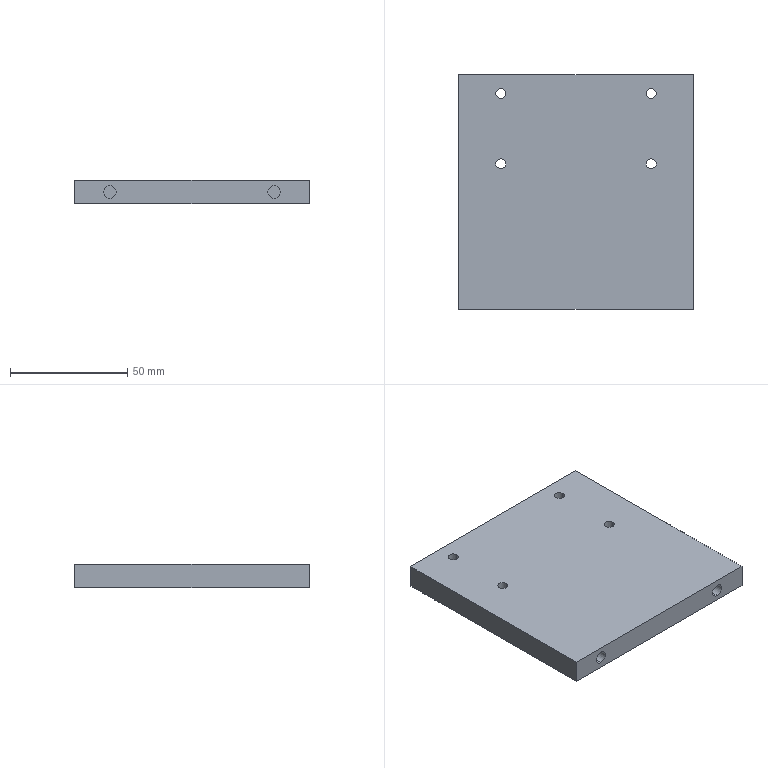Part | SolidWorks | features BaseBody 1 | 1 solid | 20 faces | box 100 x 100 x 10 mm | volume 98969 mm3 | cylinder 12 | plane 8 | commonest cylinder face diameters 4.3 x8 5.3 x4
STEP:
#1=CARTESIAN_POINT('',(34.15,42.,5.));
#2=VERTEX_POINT('',#1);
#3=CARTESIAN_POINT('',(29.85,42.,5.));
#4=VERTEX_POINT('',#3);
#5=CARTESIAN_POINT('',(32.,42.,5.));
#6=DIRECTION('',(0.,0.,-1.));
#7=DIRECTION('',(-1.,0.,0.));
#8=AXIS2_PLACEMENT_3D('',#5,#6,#7);
#9=CIRCLE('',#8,2.15);
#10=EDGE_CURVE('',#2,#4,#9,.T.);
#11=ORIENTED_EDGE('',*,*,#10,.F.);
#12=CARTESIAN_POINT('',(34.15,42.,-5.));
#13=VERTEX_POINT('',#12);
#14=CARTESIAN_POINT('',(34.15,42.,15.2));
#15=DIRECTION('',(0.,0.,-1.));
#16=VECTOR('',#15,1000.);
#17=LINE('',#14,#16);
#18=EDGE_CURVE('',#2,#13,#17,.T.);
#19=ORIENTED_EDGE('',*,*,#18,.T.);
#20=CARTESIAN_POINT('',(29.85,42.,-5.));
#21=VERTEX_POINT('',#20);
#22=CARTESIAN_POINT('',(32.,42.,-5.));
#23=DIRECTION('',(0.,0.,1.));
#24=DIRECTION('',(-1.,0.,0.));
#25=AXIS2_PLACEMENT_3D('',#22,#23,#24);
#26=CIRCLE('',#25,2.15);
#27=EDGE_CURVE('',#21,#13,#26,.T.);
#28=ORIENTED_EDGE('',*,*,#27,.F.);
#29=CARTESIAN_POINT('',(29.85,42.,15.2));
#30=DIRECTION('',(0.,0.,-1.));
#31=VECTOR('',#30,1000.);
#32=LINE('',#29,#31);
#33=EDGE_CURVE('',#4,#21,#32,.T.);
#34=ORIENTED_EDGE('',*,*,#33,.F.);
#35=EDGE_LOOP('',(#11,#19,#28,#34));
#36=FACE_OUTER_BOUND('',#35,.T.);
#37=CARTESIAN_POINT('',(32.,42.,15.2));
#38=DIRECTION('',(0.,0.,-1.));
#39=DIRECTION('',(-1.,0.,0.));
#40=AXIS2_PLACEMENT_3D('',#37,#38,#39);
#41=CYLINDRICAL_SURFACE('',#40,2.15);
#42=ADVANCED_FACE('',(#36),#41,.F.);
#43=CARTESIAN_POINT('',(-29.85,42.,5.));
#44=VERTEX_POINT('',#43);
#45=CARTESIAN_POINT('',(-34.15,42.,5.));
#46=VERTEX_POINT('',#45);
#47=CARTESIAN_POINT('',(-32.,42.,5.));
#48=DIRECTION('',(0.,0.,-1.));
#49=DIRECTION('',(-1.,0.,0.));
#50=AXIS2_PLACEMENT_3D('',#47,#48,#49);
#51=CIRCLE('',#50,2.15);
#52=EDGE_CURVE('',#44,#46,#51,.T.);
#53=ORIENTED_EDGE('',*,*,#52,.F.);
#54=CARTESIAN_POINT('',(-29.85,42.,-5.));
#55=VERTEX_POINT('',#54);
#56=CARTESIAN_POINT('',(-29.85,42.,15.2));
#57=DIRECTION('',(0.,0.,-1.));
#58=VECTOR('',#57,1000.);
#59=LINE('',#56,#58);
#60=EDGE_CURVE('',#44,#55,#59,.T.);
#61=ORIENTED_EDGE('',*,*,#60,.T.);
#62=CARTESIAN_POINT('',(-34.15,42.,-5.));
#63=VERTEX_POINT('',#62);
#64=CARTESIAN_POINT('',(-32.,42.,-5.));
#65=DIRECTION('',(0.,0.,1.));
#66=DIRECTION('',(-1.,0.,0.));
#67=AXIS2_PLACEMENT_3D('',#64,#65,#66);
#68=CIRCLE('',#67,2.15);
#69=EDGE_CURVE('',#63,#55,#68,.T.);
#70=ORIENTED_EDGE('',*,*,#69,.F.);
#71=CARTESIAN_POINT('',(-34.15,42.,15.2));
#72=DIRECTION('',(0.,0.,-1.));
#73=VECTOR('',#72,1000.);
#74=LINE('',#71,#73);
#75=EDGE_CURVE('',#46,#63,#74,.T.);
#76=ORIENTED_EDGE('',*,*,#75,.F.);
#77=EDGE_LOOP('',(#53,#61,#70,#76));
#78=FACE_OUTER_BOUND('',#77,.T.);
#79=CARTESIAN_POINT('',(-32.,42.,15.2));
#80=DIRECTION('',(0.,0.,-1.));
#81=DIRECTION('',(-1.,0.,0.));
#82=AXIS2_PLACEMENT_3D('',#79,#80,#81);
#83=CYLINDRICAL_SURFACE('',#82,2.15);
#84=ADVANCED_FACE('',(#78),#83,.F.);
#85=CARTESIAN_POINT('',(34.15,12.,5.));
#86=VERTEX_POINT('',#85);
#87=CARTESIAN_POINT('',(29.85,12.,5.));
#88=VERTEX_POINT('',#87);
#89=CARTESIAN_POINT('',(32.,12.,5.));
#90=DIRECTION('',(0.,0.,-1.));
#91=DIRECTION('',(-1.,0.,0.));
#92=AXIS2_PLACEMENT_3D('',#89,#90,#91);
#93=CIRCLE('',#92,2.15);
#94=EDGE_CURVE('',#86,#88,#93,.T.);
#95=ORIENTED_EDGE('',*,*,#94,.F.);
#96=CARTESIAN_POINT('',(34.15,12.,-5.));
#97=VERTEX_POINT('',#96);
#98=CARTESIAN_POINT('',(34.15,12.,15.2));
#99=DIRECTION('',(0.,0.,-1.));
#100=VECTOR('',#99,1000.);
#101=LINE('',#98,#100);
#102=EDGE_CURVE('',#86,#97,#101,.T.);
#103=ORIENTED_EDGE('',*,*,#102,.T.);
#104=CARTESIAN_POINT('',(29.85,12.,-5.));
#105=VERTEX_POINT('',#104);
#106=CARTESIAN_POINT('',(32.,12.,-5.));
#107=DIRECTION('',(0.,0.,1.));
#108=DIRECTION('',(-1.,0.,0.));
#109=AXIS2_PLACEMENT_3D('',#106,#107,#108);
#110=CIRCLE('',#109,2.15);
#111=EDGE_CURVE('',#105,#97,#110,.T.);
#112=ORIENTED_EDGE('',*,*,#111,.F.);
#113=CARTESIAN_POINT('',(29.85,12.,15.2));
#114=DIRECTION('',(0.,0.,-1.));
#115=VECTOR('',#114,1000.);
#116=LINE('',#113,#115);
#117=EDGE_CURVE('',#88,#105,#116,.T.);
#118=ORIENTED_EDGE('',*,*,#117,.F.);
#119=EDGE_LOOP('',(#95,#103,#112,#118));
#120=FACE_OUTER_BOUND('',#119,.T.);
#121=CARTESIAN_POINT('',(32.,12.,15.2));
#122=DIRECTION('',(0.,0.,-1.));
#123=DIRECTION('',(-1.,0.,0.));
#124=AXIS2_PLACEMENT_3D('',#121,#122,#123);
#125=CYLINDRICAL_SURFACE('',#124,2.15);
#126=ADVANCED_FACE('',(#120),#125,.F.);
#127=CARTESIAN_POINT('',(-29.85,12.,5.));
#128=VERTEX_POINT('',#127);
#129=CARTESIAN_POINT('',(-34.15,12.,5.));
#130=VERTEX_POINT('',#129);
#131=CARTESIAN_POINT('',(-32.,12.,5.));
#132=DIRECTION('',(0.,0.,-1.));
#133=DIRECTION('',(-1.,0.,0.));
#134=AXIS2_PLACEMENT_3D('',#131,#132,#133);
#135=CIRCLE('',#134,2.15);
#136=EDGE_CURVE('',#128,#130,#135,.T.);
#137=ORIENTED_EDGE('',*,*,#136,.F.);
#138=CARTESIAN_POINT('',(-29.85,12.,-5.));
#139=VERTEX_POINT('',#138);
#140=CARTESIAN_POINT('',(-29.85,12.,15.2));
#141=DIRECTION('',(0.,0.,-1.));
#142=VECTOR('',#141,1000.);
#143=LINE('',#140,#142);
#144=EDGE_CURVE('',#128,#139,#143,.T.);
#145=ORIENTED_EDGE('',*,*,#144,.T.);
#146=CARTESIAN_POINT('',(-34.15,12.,-5.));
#147=VERTEX_POINT('',#146);
#148=CARTESIAN_POINT('',(-32.,12.,-5.));
#149=DIRECTION('',(0.,0.,1.));
#150=DIRECTION('',(-1.,0.,0.));
#151=AXIS2_PLACEMENT_3D('',#148,#149,#150);
#152=CIRCLE('',#151,2.15);
#153=EDGE_CURVE('',#147,#139,#152,.T.);
#154=ORIENTED_EDGE('',*,*,#153,.F.);
#155=CARTESIAN_POINT('',(-34.15,12.,15.2));
#156=DIRECTION('',(0.,0.,-1.));
#157=VECTOR('',#156,1000.);
#158=LINE('',#155,#157);
#159=EDGE_CURVE('',#130,#147,#158,.T.);
#160=ORIENTED_EDGE('',*,*,#159,.F.);
#161=EDGE_LOOP('',(#137,#145,#154,#160));
#162=FACE_OUTER_BOUND('',#161,.T.);
#163=CARTESIAN_POINT('',(-32.,12.,15.2));
#164=DIRECTION('',(0.,0.,-1.));
#165=DIRECTION('',(-1.,0.,0.));
#166=AXIS2_PLACEMENT_3D('',#163,#164,#165);
#167=CYLINDRICAL_SURFACE('',#166,2.15);
#168=ADVANCED_FACE('',(#162),#167,.F.);
#169=CARTESIAN_POINT('',(35.,-39.8,2.65));
#170=VERTEX_POINT('',#169);
#171=CARTESIAN_POINT('',(35.,-39.8,-2.65));
#172=VERTEX_POINT('',#171);
#173=CARTESIAN_POINT('',(35.,-39.8,0.));
#174=DIRECTION('',(0.,-1.,0.));
#175=DIRECTION('',(0.,0.,-1.));
#176=AXIS2_PLACEMENT_3D('',#173,#174,#175);
#177=CIRCLE('',#176,2.65);
#178=EDGE_CURVE('',#170,#172,#177,.T.);
#179=ORIENTED_EDGE('',*,*,#178,.F.);
#180=CARTESIAN_POINT('',(35.,-50.,2.65));
#181=VERTEX_POINT('',#180);
#182=CARTESIAN_POINT('',(35.,-39.8,2.65));
#183=DIRECTION('',(0.,-1.,0.));
#184=VECTOR('',#183,1000.);
#185=LINE('',#182,#184);
#186=EDGE_CURVE('',#170,#181,#185,.T.);
#187=ORIENTED_EDGE('',*,*,#186,.T.);
#188=CARTESIAN_POINT('',(35.,-50.,-2.65));
#189=VERTEX_POINT('',#188);
#190=CARTESIAN_POINT('',(35.,-50.,0.));
#191=DIRECTION('',(0.,-1.,0.));
#192=DIRECTION('',(0.,0.,-1.));
#193=AXIS2_PLACEMENT_3D('',#190,#191,#192);
#194=CIRCLE('',#193,2.65);
#195=EDGE_CURVE('',#181,#189,#194,.T.);
#196=ORIENTED_EDGE('',*,*,#195,.T.);
#197=CARTESIAN_POINT('',(35.,-39.8,-2.65));
#198=DIRECTION('',(0.,-1.,0.));
#199=VECTOR('',#198,1000.);
#200=LINE('',#197,#199);
#201=EDGE_CURVE('',#172,#189,#200,.T.);
#202=ORIENTED_EDGE('',*,*,#201,.F.);
#203=EDGE_LOOP('',(#179,#187,#196,#202));
#204=FACE_OUTER_BOUND('',#203,.T.);
#205=CARTESIAN_POINT('',(35.,-39.8,0.));
#206=DIRECTION('',(0.,-1.,0.));
#207=DIRECTION('',(0.,0.,-1.));
#208=AXIS2_PLACEMENT_3D('',#205,#206,#207);
#209=CYLINDRICAL_SURFACE('',#208,2.65);
#210=ADVANCED_FACE('',(#204),#209,.F.);
#211=CARTESIAN_POINT('',(-35.,-39.8,2.65));
#212=VERTEX_POINT('',#211);
#213=CARTESIAN_POINT('',(-35.,-39.8,-2.65));
#214=VERTEX_POINT('',#213);
#215=CARTESIAN_POINT('',(-35.,-39.8,0.));
#216=DIRECTION('',(0.,-1.,0.));
#217=DIRECTION('',(0.,0.,-1.));
#218=AXIS2_PLACEMENT_3D('',#215,#216,#217);
#219=CIRCLE('',#218,2.65);
#220=EDGE_CURVE('',#212,#214,#219,.T.);
#221=ORIENTED_EDGE('',*,*,#220,.F.);
#222=CARTESIAN_POINT('',(-35.,-50.,2.65));
#223=VERTEX_POINT('',#222);
#224=CARTESIAN_POINT('',(-35.,-39.8,2.65));
#225=DIRECTION('',(0.,-1.,0.));
#226=VECTOR('',#225,1000.);
#227=LINE('',#224,#226);
#228=EDGE_CURVE('',#212,#223,#227,.T.);
#229=ORIENTED_EDGE('',*,*,#228,.T.);
#230=CARTESIAN_POINT('',(-35.,-50.,-2.65));
#231=VERTEX_POINT('',#230);
#232=CARTESIAN_POINT('',(-35.,-50.,0.));
#233=DIRECTION('',(0.,-1.,0.));
#234=DIRECTION('',(0.,0.,-1.));
#235=AXIS2_PLACEMENT_3D('',#232,#233,#234);
#236=CIRCLE('',#235,2.65);
#237=EDGE_CURVE('',#223,#231,#236,.T.);
#238=ORIENTED_EDGE('',*,*,#237,.T.);
#239=CARTESIAN_POINT('',(-35.,-39.8,-2.65));
#240=DIRECTION('',(0.,-1.,0.));
#241=VECTOR('',#240,1000.);
#242=LINE('',#239,#241);
#243=EDGE_CURVE('',#214,#231,#242,.T.);
#244=ORIENTED_EDGE('',*,*,#243,.F.);
#245=EDGE_LOOP('',(#221,#229,#238,#244));
#246=FACE_OUTER_BOUND('',#245,.T.);
#247=CARTESIAN_POINT('',(-35.,-39.8,0.));
#248=DIRECTION('',(0.,-1.,0.));
#249=DIRECTION('',(0.,0.,-1.));
#250=AXIS2_PLACEMENT_3D('',#247,#248,#249);
#251=CYLINDRICAL_SURFACE('',#250,2.65);
#252=ADVANCED_FACE('',(#246),#251,.F.);
#253=CARTESIAN_POINT('',(32.,42.,5.));
#254=DIRECTION('',(0.,0.,-1.));
#255=DIRECTION('',(-1.,0.,0.));
#256=AXIS2_PLACEMENT_3D('',#253,#254,#255);
#257=CIRCLE('',#256,2.15);
#258=EDGE_CURVE('',#4,#2,#257,.T.);
#259=ORIENTED_EDGE('',*,*,#258,.T.);
#260=ORIENTED_EDGE('',*,*,#10,.T.);
#261=EDGE_LOOP('',(#259,#260));
#262=FACE_BOUND('',#261,.T.);
#263=CARTESIAN_POINT('',(-32.,42.,5.));
#264=DIRECTION('',(0.,0.,-1.));
#265=DIRECTION('',(-1.,0.,0.));
#266=AXIS2_PLACEMENT_3D('',#263,#264,#265);
#267=CIRCLE('',#266,2.15);
#268=EDGE_CURVE('',#46,#44,#267,.T.);
#269=ORIENTED_EDGE('',*,*,#268,.T.);
#270=ORIENTED_EDGE('',*,*,#52,.T.);
#271=EDGE_LOOP('',(#269,#270));
#272=FACE_BOUND('',#271,.T.);
#273=CARTESIAN_POINT('',(32.,12.,5.));
#274=DIRECTION('',(0.,0.,-1.));
#275=DIRECTION('',(-1.,0.,0.));
#276=AXIS2_PLACEMENT_3D('',#273,#274,#275);
#277=CIRCLE('',#276,2.15);
#278=EDGE_CURVE('',#88,#86,#277,.T.);
#279=ORIENTED_EDGE('',*,*,#278,.T.);
#280=ORIENTED_EDGE('',*,*,#94,.T.);
#281=EDGE_LOOP('',(#279,#280));
#282=FACE_BOUND('',#281,.T.);
#283=CARTESIAN_POINT('',(-32.,12.,5.));
#284=DIRECTION('',(0.,0.,-1.));
#285=DIRECTION('',(-1.,0.,0.));
#286=AXIS2_PLACEMENT_3D('',#283,#284,#285);
#287=CIRCLE('',#286,2.15);
#288=EDGE_CURVE('',#130,#128,#287,.T.);
#289=ORIENTED_EDGE('',*,*,#288,.T.);
#290=ORIENTED_EDGE('',*,*,#136,.T.);
#291=EDGE_LOOP('',(#289,#290));
#292=FACE_BOUND('',#291,.T.);
#293=CARTESIAN_POINT('',(50.,-50.,5.));
#294=VERTEX_POINT('',#293);
#295=CARTESIAN_POINT('',(50.,50.,5.));
#296=VERTEX_POINT('',#295);
#297=CARTESIAN_POINT('',(50.,-50.,5.));
#298=DIRECTION('',(0.,1.,0.));
#299=VECTOR('',#298,1000.);
#300=LINE('',#297,#299);
#301=EDGE_CURVE('',#294,#296,#300,.T.);
#302=ORIENTED_EDGE('',*,*,#301,.T.);
#303=CARTESIAN_POINT('',(-50.,50.,5.));
#304=VERTEX_POINT('',#303);
#305=CARTESIAN_POINT('',(-50.,50.,5.));
#306=DIRECTION('',(-1.,0.,0.));
#307=VECTOR('',#306,1000.);
#308=LINE('',#305,#307);
#309=EDGE_CURVE('',#296,#304,#308,.T.);
#310=ORIENTED_EDGE('',*,*,#309,.T.);
#311=CARTESIAN_POINT('',(-50.,-50.,5.));
#312=VERTEX_POINT('',#311);
#313=CARTESIAN_POINT('',(-50.,-50.,5.));
#314=DIRECTION('',(0.,-1.,0.));
#315=VECTOR('',#314,1000.);
#316=LINE('',#313,#315);
#317=EDGE_CURVE('',#304,#312,#316,.T.);
#318=ORIENTED_EDGE('',*,*,#317,.T.);
#319=CARTESIAN_POINT('',(-50.,-50.,5.));
#320=DIRECTION('',(1.,0.,0.));
#321=VECTOR('',#320,1000.);
#322=LINE('',#319,#321);
#323=EDGE_CURVE('',#312,#294,#322,.T.);
#324=ORIENTED_EDGE('',*,*,#323,.T.);
#325=EDGE_LOOP('',(#302,#310,#318,#324));
#326=FACE_OUTER_BOUND('',#325,.T.);
#327=CARTESIAN_POINT('',(-50.,-50.,5.));
#328=DIRECTION('',(0.,0.,1.));
#329=DIRECTION('',(1.,0.,0.));
#330=AXIS2_PLACEMENT_3D('',#327,#328,#329);
#331=PLANE('',#330);
#332=ADVANCED_FACE('',(#262,#272,#282,#292,#326),#331,.T.);
#333=ORIENTED_EDGE('',*,*,#18,.F.);
#334=ORIENTED_EDGE('',*,*,#258,.F.);
#335=ORIENTED_EDGE('',*,*,#33,.T.);
#336=CARTESIAN_POINT('',(32.,42.,-5.));
#337=DIRECTION('',(0.,0.,1.));
#338=DIRECTION('',(-1.,0.,0.));
#339=AXIS2_PLACEMENT_3D('',#336,#337,#338);
#340=CIRCLE('',#339,2.15);
#341=EDGE_CURVE('',#13,#21,#340,.T.);
#342=ORIENTED_EDGE('',*,*,#341,.F.);
#343=EDGE_LOOP('',(#333,#334,#335,#342));
#344=FACE_OUTER_BOUND('',#343,.T.);
#345=CARTESIAN_POINT('',(32.,42.,15.2));
#346=DIRECTION('',(0.,0.,-1.));
#347=DIRECTION('',(-1.,0.,0.));
#348=AXIS2_PLACEMENT_3D('',#345,#346,#347);
#349=CYLINDRICAL_SURFACE('',#348,2.15);
#350=ADVANCED_FACE('',(#344),#349,.F.);
#351=ORIENTED_EDGE('',*,*,#60,.F.);
#352=ORIENTED_EDGE('',*,*,#268,.F.);
#353=ORIENTED_EDGE('',*,*,#75,.T.);
#354=CARTESIAN_POINT('',(-32.,42.,-5.));
#355=DIRECTION('',(0.,0.,1.));
#356=DIRECTION('',(-1.,0.,0.));
#357=AXIS2_PLACEMENT_3D('',#354,#355,#356);
#358=CIRCLE('',#357,2.15);
#359=EDGE_CURVE('',#55,#63,#358,.T.);
#360=ORIENTED_EDGE('',*,*,#359,.F.);
#361=EDGE_LOOP('',(#351,#352,#353,#360));
#362=FACE_OUTER_BOUND('',#361,.T.);
#363=CARTESIAN_POINT('',(-32.,42.,15.2));
#364=DIRECTION('',(0.,0.,-1.));
#365=DIRECTION('',(-1.,0.,0.));
#366=AXIS2_PLACEMENT_3D('',#363,#364,#365);
#367=CYLINDRICAL_SURFACE('',#366,2.15);
#368=ADVANCED_FACE('',(#362),#367,.F.);
#369=ORIENTED_EDGE('',*,*,#102,.F.);
#370=ORIENTED_EDGE('',*,*,#278,.F.);
#371=ORIENTED_EDGE('',*,*,#117,.T.);
#372=CARTESIAN_POINT('',(32.,12.,-5.));
#373=DIRECTION('',(0.,0.,1.));
#374=DIRECTION('',(-1.,0.,0.));
#375=AXIS2_PLACEMENT_3D('',#372,#373,#374);
#376=CIRCLE('',#375,2.15);
#377=EDGE_CURVE('',#97,#105,#376,.T.);
#378=ORIENTED_EDGE('',*,*,#377,.F.);
#379=EDGE_LOOP('',(#369,#370,#371,#378));
#380=FACE_OUTER_BOUND('',#379,.T.);
#381=CARTESIAN_POINT('',(32.,12.,15.2));
#382=DIRECTION('',(0.,0.,-1.));
#383=DIRECTION('',(-1.,0.,0.));
#384=AXIS2_PLACEMENT_3D('',#381,#382,#383);
#385=CYLINDRICAL_SURFACE('',#384,2.15);
#386=ADVANCED_FACE('',(#380),#385,.F.);
#387=ORIENTED_EDGE('',*,*,#144,.F.);
#388=ORIENTED_EDGE('',*,*,#288,.F.);
#389=ORIENTED_EDGE('',*,*,#159,.T.);
#390=CARTESIAN_POINT('',(-32.,12.,-5.));
#391=DIRECTION('',(0.,0.,1.));
#392=DIRECTION('',(-1.,0.,0.));
#393=AXIS2_PLACEMENT_3D('',#390,#391,#392);
#394=CIRCLE('',#393,2.15);
#395=EDGE_CURVE('',#139,#147,#394,.T.);
#396=ORIENTED_EDGE('',*,*,#395,.F.);
#397=EDGE_LOOP('',(#387,#388,#389,#396));
#398=FACE_OUTER_BOUND('',#397,.T.);
#399=CARTESIAN_POINT('',(-32.,12.,15.2));
#400=DIRECTION('',(0.,0.,-1.));
#401=DIRECTION('',(-1.,0.,0.));
#402=AXIS2_PLACEMENT_3D('',#399,#400,#401);
#403=CYLINDRICAL_SURFACE('',#402,2.15);
#404=ADVANCED_FACE('',(#398),#403,.F.);
#405=ORIENTED_EDGE('',*,*,#309,.F.);
#406=CARTESIAN_POINT('',(50.,50.,-5.));
#407=VERTEX_POINT('',#406);
#408=CARTESIAN_POINT('',(50.,50.,-5.));
#409=DIRECTION('',(0.,0.,-1.));
#410=VECTOR('',#409,1000.);
#411=LINE('',#408,#410);
#412=EDGE_CURVE('',#296,#407,#411,.T.);
#413=ORIENTED_EDGE('',*,*,#412,.T.);
#414=CARTESIAN_POINT('',(-50.,50.,-5.));
#415=VERTEX_POINT('',#414);
#416=CARTESIAN_POINT('',(-50.,50.,-5.));
#417=DIRECTION('',(-1.,0.,0.));
#418=VECTOR('',#417,1000.);
#419=LINE('',#416,#418);
#420=EDGE_CURVE('',#407,#415,#419,.T.);
#421=ORIENTED_EDGE('',*,*,#420,.T.);
#422=CARTESIAN_POINT('',(-50.,50.,-5.));
#423=DIRECTION('',(0.,0.,1.));
#424=VECTOR('',#423,1000.);
#425=LINE('',#422,#424);
#426=EDGE_CURVE('',#415,#304,#425,.T.);
#427=ORIENTED_EDGE('',*,*,#426,.T.);
#428=EDGE_LOOP('',(#405,#413,#421,#427));
#429=FACE_OUTER_BOUND('',#428,.T.);
#430=CARTESIAN_POINT('',(-50.,50.,-5.));
#431=DIRECTION('',(0.,1.,0.));
#432=DIRECTION('',(0.,0.,1.));
#433=AXIS2_PLACEMENT_3D('',#430,#431,#432);
#434=PLANE('',#433);
#435=ADVANCED_FACE('',(#429),#434,.T.);
#436=ORIENTED_EDGE('',*,*,#412,.F.);
#437=ORIENTED_EDGE('',*,*,#301,.F.);
#438=CARTESIAN_POINT('',(50.,-50.,-5.));
#439=VERTEX_POINT('',#438);
#440=CARTESIAN_POINT('',(50.,-50.,-5.));
#441=DIRECTION('',(0.,0.,-1.));
#442=VECTOR('',#441,1000.);
#443=LINE('',#440,#442);
#444=EDGE_CURVE('',#294,#439,#443,.T.);
#445=ORIENTED_EDGE('',*,*,#444,.T.);
#446=CARTESIAN_POINT('',(50.,-50.,-5.));
#447=DIRECTION('',(0.,1.,0.));
#448=VECTOR('',#447,1000.);
#449=LINE('',#446,#448);
#450=EDGE_CURVE('',#439,#407,#449,.T.);
#451=ORIENTED_EDGE('',*,*,#450,.T.);
#452=EDGE_LOOP('',(#436,#437,#445,#451));
#453=FACE_OUTER_BOUND('',#452,.T.);
#454=CARTESIAN_POINT('',(50.,-50.,-5.));
#455=DIRECTION('',(1.,0.,0.));
#456=DIRECTION('',(0.,0.,-1.));
#457=AXIS2_PLACEMENT_3D('',#454,#455,#456);
#458=PLANE('',#457);
#459=ADVANCED_FACE('',(#453),#458,.T.);
#460=CARTESIAN_POINT('',(35.,-50.,0.));
#461=DIRECTION('',(0.,-1.,0.));
#462=DIRECTION('',(0.,0.,-1.));
#463=AXIS2_PLACEMENT_3D('',#460,#461,#462);
#464=CIRCLE('',#463,2.65);
#465=EDGE_CURVE('',#189,#181,#464,.T.);
#466=ORIENTED_EDGE('',*,*,#465,.F.);
#467=ORIENTED_EDGE('',*,*,#195,.F.);
#468=EDGE_LOOP('',(#466,#467));
#469=FACE_BOUND('',#468,.T.);
#470=CARTESIAN_POINT('',(-35.,-50.,0.));
#471=DIRECTION('',(0.,-1.,0.));
#472=DIRECTION('',(0.,0.,-1.));
#473=AXIS2_PLACEMENT_3D('',#470,#471,#472);
#474=CIRCLE('',#473,2.65);
#475=EDGE_CURVE('',#231,#223,#474,.T.);
#476=ORIENTED_EDGE('',*,*,#475,.F.);
#477=ORIENTED_EDGE('',*,*,#237,.F.);
#478=EDGE_LOOP('',(#476,#477));
#479=FACE_BOUND('',#478,.T.);
#480=ORIENTED_EDGE('',*,*,#323,.F.);
#481=CARTESIAN_POINT('',(-50.,-50.,-5.));
#482=VERTEX_POINT('',#481);
#483=CARTESIAN_POINT('',(-50.,-50.,-5.));
#484=DIRECTION('',(0.,0.,1.));
#485=VECTOR('',#484,1000.);
#486=LINE('',#483,#485);
#487=EDGE_CURVE('',#482,#312,#486,.T.);
#488=ORIENTED_EDGE('',*,*,#487,.F.);
#489=CARTESIAN_POINT('',(-50.,-50.,-5.));
#490=DIRECTION('',(-1.,0.,0.));
#491=VECTOR('',#490,1000.);
#492=LINE('',#489,#491);
#493=EDGE_CURVE('',#439,#482,#492,.T.);
#494=ORIENTED_EDGE('',*,*,#493,.F.);
#495=ORIENTED_EDGE('',*,*,#444,.F.);
#496=EDGE_LOOP('',(#480,#488,#494,#495));
#497=FACE_OUTER_BOUND('',#496,.T.);
#498=CARTESIAN_POINT('',(-50.,-50.,-5.));
#499=DIRECTION('',(0.,1.,0.));
#500=DIRECTION('',(0.,0.,1.));
#501=AXIS2_PLACEMENT_3D('',#498,#499,#500);
#502=PLANE('',#501);
#503=ADVANCED_FACE('',(#469,#479,#497),#502,.F.);
#504=ORIENTED_EDGE('',*,*,#426,.F.);
#505=CARTESIAN_POINT('',(-50.,-50.,-5.));
#506=DIRECTION('',(0.,1.,0.));
#507=VECTOR('',#506,1000.);
#508=LINE('',#505,#507);
#509=EDGE_CURVE('',#482,#415,#508,.T.);
#510=ORIENTED_EDGE('',*,*,#509,.F.);
#511=ORIENTED_EDGE('',*,*,#487,.T.);
#512=ORIENTED_EDGE('',*,*,#317,.F.);
#513=EDGE_LOOP('',(#504,#510,#511,#512));
#514=FACE_OUTER_BOUND('',#513,.T.);
#515=CARTESIAN_POINT('',(-50.,-50.,-5.));
#516=DIRECTION('',(1.,0.,0.));
#517=DIRECTION('',(0.,0.,-1.));
#518=AXIS2_PLACEMENT_3D('',#515,#516,#517);
#519=PLANE('',#518);
#520=ADVANCED_FACE('',(#514),#519,.F.);
#521=ORIENTED_EDGE('',*,*,#27,.T.);
#522=ORIENTED_EDGE('',*,*,#341,.T.);
#523=EDGE_LOOP('',(#521,#522));
#524=FACE_BOUND('',#523,.T.);
#525=ORIENTED_EDGE('',*,*,#69,.T.);
#526=ORIENTED_EDGE('',*,*,#359,.T.);
#527=EDGE_LOOP('',(#525,#526));
#528=FACE_BOUND('',#527,.T.);
#529=ORIENTED_EDGE('',*,*,#111,.T.);
#530=ORIENTED_EDGE('',*,*,#377,.T.);
#531=EDGE_LOOP('',(#529,#530));
#532=FACE_BOUND('',#531,.T.);
#533=ORIENTED_EDGE('',*,*,#153,.T.);
#534=ORIENTED_EDGE('',*,*,#395,.T.);
#535=EDGE_LOOP('',(#533,#534));
#536=FACE_BOUND('',#535,.T.);
#537=ORIENTED_EDGE('',*,*,#450,.F.);
#538=ORIENTED_EDGE('',*,*,#493,.T.);
#539=ORIENTED_EDGE('',*,*,#509,.T.);
#540=ORIENTED_EDGE('',*,*,#420,.F.);
#541=EDGE_LOOP('',(#537,#538,#539,#540));
#542=FACE_OUTER_BOUND('',#541,.T.);
#543=CARTESIAN_POINT('',(-50.,-50.,-5.));
#544=DIRECTION('',(0.,0.,1.));
#545=DIRECTION('',(1.,0.,0.));
#546=AXIS2_PLACEMENT_3D('',#543,#544,#545);
#547=PLANE('',#546);
#548=ADVANCED_FACE('',(#524,#528,#532,#536,#542),#547,.F.);
#549=ORIENTED_EDGE('',*,*,#186,.F.);
#550=CARTESIAN_POINT('',(35.,-39.8,0.));
#551=DIRECTION('',(0.,-1.,0.));
#552=DIRECTION('',(0.,0.,-1.));
#553=AXIS2_PLACEMENT_3D('',#550,#551,#552);
#554=CIRCLE('',#553,2.65);
#555=EDGE_CURVE('',#172,#170,#554,.T.);
#556=ORIENTED_EDGE('',*,*,#555,.F.);
#557=ORIENTED_EDGE('',*,*,#201,.T.);
#558=ORIENTED_EDGE('',*,*,#465,.T.);
#559=EDGE_LOOP('',(#549,#556,#557,#558));
#560=FACE_OUTER_BOUND('',#559,.T.);
#561=CARTESIAN_POINT('',(35.,-39.8,0.));
#562=DIRECTION('',(0.,-1.,0.));
#563=DIRECTION('',(0.,0.,-1.));
#564=AXIS2_PLACEMENT_3D('',#561,#562,#563);
#565=CYLINDRICAL_SURFACE('',#564,2.65);
#566=ADVANCED_FACE('',(#560),#565,.F.);
#567=ORIENTED_EDGE('',*,*,#228,.F.);
#568=CARTESIAN_POINT('',(-35.,-39.8,0.));
#569=DIRECTION('',(0.,-1.,0.));
#570=DIRECTION('',(0.,0.,-1.));
#571=AXIS2_PLACEMENT_3D('',#568,#569,#570);
#572=CIRCLE('',#571,2.65);
#573=EDGE_CURVE('',#214,#212,#572,.T.);
#574=ORIENTED_EDGE('',*,*,#573,.F.);
#575=ORIENTED_EDGE('',*,*,#243,.T.);
#576=ORIENTED_EDGE('',*,*,#475,.T.);
#577=EDGE_LOOP('',(#567,#574,#575,#576));
#578=FACE_OUTER_BOUND('',#577,.T.);
#579=CARTESIAN_POINT('',(-35.,-39.8,0.));
#580=DIRECTION('',(0.,-1.,0.));
#581=DIRECTION('',(0.,0.,-1.));
#582=AXIS2_PLACEMENT_3D('',#579,#580,#581);
#583=CYLINDRICAL_SURFACE('',#582,2.65);
#584=ADVANCED_FACE('',(#578),#583,.F.);
#585=ORIENTED_EDGE('',*,*,#555,.T.);
#586=ORIENTED_EDGE('',*,*,#178,.T.);
#587=EDGE_LOOP('',(#585,#586));
#588=FACE_OUTER_BOUND('',#587,.T.);
#589=CARTESIAN_POINT('',(35.,-39.8,0.));
#590=DIRECTION('',(0.,-1.,0.));
#591=DIRECTION('',(0.,0.,-1.));
#592=AXIS2_PLACEMENT_3D('',#589,#590,#591);
#593=PLANE('',#592);
#594=ADVANCED_FACE('',(#588),#593,.T.);
#595=ORIENTED_EDGE('',*,*,#573,.T.);
#596=ORIENTED_EDGE('',*,*,#220,.T.);
#597=EDGE_LOOP('',(#595,#596));
#598=FACE_OUTER_BOUND('',#597,.T.);
#599=CARTESIAN_POINT('',(-35.,-39.8,0.));
#600=DIRECTION('',(0.,-1.,0.));
#601=DIRECTION('',(0.,0.,-1.));
#602=AXIS2_PLACEMENT_3D('',#599,#600,#601);
#603=PLANE('',#602);
#604=ADVANCED_FACE('',(#598),#603,.T.);
#605=CLOSED_SHELL('',(#42,#84,#126,#168,#210,#252,#332,#350,#368,#386,#404,#435,#459,#503,#520,#548,#566,#584,#594,#604));
#606=MANIFOLD_SOLID_BREP('',#605);
#607=CARTESIAN_POINT('',(0.,0.,0.));
#608=DIRECTION('',(0.,0.,1.));
#609=DIRECTION('',(1.,0.,0.));
#610=AXIS2_PLACEMENT_3D('',#607,#608,#609);
#611=(LENGTH_UNIT()NAMED_UNIT(*)SI_UNIT(.MILLI.,.METRE.));
#612=UNCERTAINTY_MEASURE_WITH_UNIT(LENGTH_MEASURE(0.00001),#611,'','');
#613=(NAMED_UNIT(*)PLANE_ANGLE_UNIT()SI_UNIT($,.RADIAN.));
#614=(NAMED_UNIT(*)SI_UNIT($,.STERADIAN.)SOLID_ANGLE_UNIT());
#615=(GEOMETRIC_REPRESENTATION_CONTEXT(3)GLOBAL_UNCERTAINTY_ASSIGNED_CONTEXT((#612))GLOBAL_UNIT_ASSIGNED_CONTEXT((#611,#613,#614))REPRESENTATION_CONTEXT('',''));
#616=ADVANCED_BREP_SHAPE_REPRESENTATION('',(#606,#610),#615);